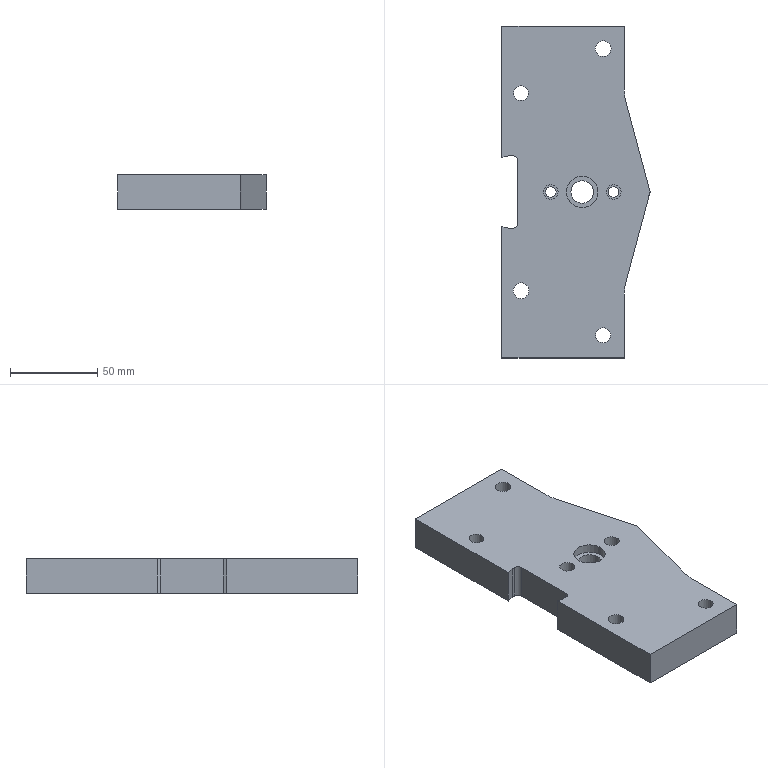Part | NX | features solid 2 | 1 solid | 40 faces | box 84.759 x 190 x 20 mm | volume 261457 mm3 | plane 22 | cylinder 18 | commonest cylinder face diameters 8.5 x4 14 x4 6 x2 6.1 x2 9 x2 52 x2
STEP:
#1=CARTESIAN_POINT('',(1132.061,-95.,20.));
#2=VERTEX_POINT('',#1);
#3=CARTESIAN_POINT('',(1132.061,-19.773,20.));
#4=VERTEX_POINT('',#3);
#5=CARTESIAN_POINT('',(1132.061,-128.277,20.));
#6=DIRECTION('',(0.,1.,0.));
#7=VECTOR('',#6,1000.);
#8=LINE('',#5,#7);
#9=EDGE_CURVE('',#2,#4,#8,.T.);
#10=ORIENTED_EDGE('',*,*,#9,.T.);
#11=CARTESIAN_POINT('',(1132.061,-19.773,0.));
#12=VERTEX_POINT('',#11);
#13=CARTESIAN_POINT('',(1132.061,-19.773,0.));
#14=DIRECTION('',(0.,0.,1.));
#15=VECTOR('',#14,1000.);
#16=LINE('',#13,#15);
#17=EDGE_CURVE('',#4,#12,#16,.F.);
#18=ORIENTED_EDGE('',*,*,#17,.T.);
#19=CARTESIAN_POINT('',(1132.061,-95.,0.));
#20=VERTEX_POINT('',#19);
#21=CARTESIAN_POINT('',(1132.061,1232.968,0.));
#22=DIRECTION('',(0.,-1.,0.));
#23=VECTOR('',#22,1000.);
#24=LINE('',#21,#23);
#25=EDGE_CURVE('',#20,#12,#24,.F.);
#26=ORIENTED_EDGE('',*,*,#25,.F.);
#27=CARTESIAN_POINT('',(1132.061,-95.,0.));
#28=DIRECTION('',(0.,0.,-1.));
#29=VECTOR('',#28,1000.);
#30=LINE('',#27,#29);
#31=EDGE_CURVE('',#20,#2,#30,.F.);
#32=ORIENTED_EDGE('',*,*,#31,.T.);
#33=EDGE_LOOP('',(#10,#18,#26,#32));
#34=FACE_BOUND('',#33,.T.);
#35=CARTESIAN_POINT('',(1132.061,-4.006,0.));
#36=DIRECTION('',(1.,0.,0.));
#37=DIRECTION('',(0.,0.,-1.));
#38=AXIS2_PLACEMENT_3D('',#35,#36,#37);
#39=PLANE('',#38);
#40=ADVANCED_FACE('',(#34),#39,.F.);
#41=CARTESIAN_POINT('',(1132.061,19.773,0.));
#42=VERTEX_POINT('',#41);
#43=CARTESIAN_POINT('',(1132.061,95.,0.));
#44=VERTEX_POINT('',#43);
#45=CARTESIAN_POINT('',(1132.061,1232.968,0.));
#46=DIRECTION('',(0.,-1.,0.));
#47=VECTOR('',#46,1000.);
#48=LINE('',#45,#47);
#49=EDGE_CURVE('',#42,#44,#48,.F.);
#50=ORIENTED_EDGE('',*,*,#49,.F.);
#51=CARTESIAN_POINT('',(1132.061,19.773,20.));
#52=VERTEX_POINT('',#51);
#53=CARTESIAN_POINT('',(1132.061,19.773,0.));
#54=DIRECTION('',(0.,0.,-1.));
#55=VECTOR('',#54,1000.);
#56=LINE('',#53,#55);
#57=EDGE_CURVE('',#42,#52,#56,.F.);
#58=ORIENTED_EDGE('',*,*,#57,.T.);
#59=CARTESIAN_POINT('',(1132.061,95.,20.));
#60=VERTEX_POINT('',#59);
#61=CARTESIAN_POINT('',(1132.061,-128.277,20.));
#62=DIRECTION('',(0.,1.,0.));
#63=VECTOR('',#62,1000.);
#64=LINE('',#61,#63);
#65=EDGE_CURVE('',#52,#60,#64,.T.);
#66=ORIENTED_EDGE('',*,*,#65,.T.);
#67=CARTESIAN_POINT('',(1132.061,95.,0.));
#68=DIRECTION('',(0.,0.,1.));
#69=VECTOR('',#68,1000.);
#70=LINE('',#67,#69);
#71=EDGE_CURVE('',#60,#44,#70,.F.);
#72=ORIENTED_EDGE('',*,*,#71,.T.);
#73=EDGE_LOOP('',(#50,#58,#66,#72));
#74=FACE_BOUND('',#73,.T.);
#75=CARTESIAN_POINT('',(1132.061,-4.006,0.));
#76=DIRECTION('',(1.,0.,0.));
#77=DIRECTION('',(0.,0.,-1.));
#78=AXIS2_PLACEMENT_3D('',#75,#76,#77);
#79=PLANE('',#78);
#80=ADVANCED_FACE('',(#74),#79,.F.);
#81=CARTESIAN_POINT('',(1196.995,-82.024,0.00000121));
#82=VERTEX_POINT('',#81);
#83=CARTESIAN_POINT('',(1189.995,-82.024,0.00000121));
#84=DIRECTION('',(0.,0.,1.));
#85=DIRECTION('',(1.,0.,0.));
#86=AXIS2_PLACEMENT_3D('',#83,#84,#85);
#87=CIRCLE('',#86,7.);
#88=EDGE_CURVE('',#82,#82,#87,.T.);
#89=ORIENTED_EDGE('',*,*,#88,.T.);
#90=EDGE_LOOP('',(#89));
#91=FACE_BOUND('',#90,.T.);
#92=CARTESIAN_POINT('',(1149.995,-56.54,0.00000121));
#93=VERTEX_POINT('',#92);
#94=CARTESIAN_POINT('',(1142.995,-56.54,0.00000121));
#95=DIRECTION('',(0.,0.,1.));
#96=DIRECTION('',(1.,0.,0.));
#97=AXIS2_PLACEMENT_3D('',#94,#95,#96);
#98=CIRCLE('',#97,7.);
#99=EDGE_CURVE('',#93,#93,#98,.T.);
#100=ORIENTED_EDGE('',*,*,#99,.T.);
#101=EDGE_LOOP('',(#100));
#102=FACE_BOUND('',#101,.T.);
#103=CARTESIAN_POINT('',(1149.995,56.54,0.00000121));
#104=VERTEX_POINT('',#103);
#105=CARTESIAN_POINT('',(1142.995,56.54,0.00000121));
#106=DIRECTION('',(0.,0.,-1.));
#107=DIRECTION('',(1.,0.,0.));
#108=AXIS2_PLACEMENT_3D('',#105,#106,#107);
#109=CIRCLE('',#108,7.);
#110=EDGE_CURVE('',#104,#104,#109,.F.);
#111=ORIENTED_EDGE('',*,*,#110,.T.);
#112=EDGE_LOOP('',(#111));
#113=FACE_BOUND('',#112,.T.);
#114=CARTESIAN_POINT('',(1196.995,82.024,0.00000121));
#115=VERTEX_POINT('',#114);
#116=CARTESIAN_POINT('',(1189.995,82.024,0.00000121));
#117=DIRECTION('',(0.,0.,-1.));
#118=DIRECTION('',(1.,0.,0.));
#119=AXIS2_PLACEMENT_3D('',#116,#117,#118);
#120=CIRCLE('',#119,7.);
#121=EDGE_CURVE('',#115,#115,#120,.F.);
#122=ORIENTED_EDGE('',*,*,#121,.T.);
#123=EDGE_LOOP('',(#122));
#124=FACE_BOUND('',#123,.T.);
#125=CARTESIAN_POINT('',(1156.95,0.,0.));
#126=VERTEX_POINT('',#125);
#127=CARTESIAN_POINT('',(1160.,0.,0.));
#128=DIRECTION('',(0.,0.,-1.));
#129=DIRECTION('',(-1.,0.,0.));
#130=AXIS2_PLACEMENT_3D('',#127,#128,#129);
#131=CIRCLE('',#130,3.05);
#132=EDGE_CURVE('',#126,#126,#131,.F.);
#133=ORIENTED_EDGE('',*,*,#132,.T.);
#134=EDGE_LOOP('',(#133));
#135=FACE_BOUND('',#134,.T.);
#136=CARTESIAN_POINT('',(1192.95,0.,0.));
#137=VERTEX_POINT('',#136);
#138=CARTESIAN_POINT('',(1196.,0.,0.));
#139=DIRECTION('',(0.,0.,-1.));
#140=DIRECTION('',(-1.,0.,0.));
#141=AXIS2_PLACEMENT_3D('',#138,#139,#140);
#142=CIRCLE('',#141,3.05);
#143=EDGE_CURVE('',#137,#137,#142,.F.);
#144=ORIENTED_EDGE('',*,*,#143,.T.);
#145=EDGE_LOOP('',(#144));
#146=FACE_BOUND('',#145,.T.);
#147=CARTESIAN_POINT('',(1171.5,0.,0.));
#148=VERTEX_POINT('',#147);
#149=CARTESIAN_POINT('',(1178.,0.,0.));
#150=DIRECTION('',(0.,0.,-1.));
#151=DIRECTION('',(-1.,0.,0.));
#152=AXIS2_PLACEMENT_3D('',#149,#150,#151);
#153=CIRCLE('',#152,6.5);
#154=EDGE_CURVE('',#148,#148,#153,.T.);
#155=ORIENTED_EDGE('',*,*,#154,.F.);
#156=EDGE_LOOP('',(#155));
#157=FACE_BOUND('',#156,.T.);
#158=CARTESIAN_POINT('',(1138.074,20.88,0.));
#159=VERTEX_POINT('',#158);
#160=CARTESIAN_POINT('',(1136.159,20.88,0.));
#161=VERTEX_POINT('',#160);
#162=CARTESIAN_POINT('',(178.557,20.88,0.));
#163=DIRECTION('',(-1.,0.,0.));
#164=VECTOR('',#163,1000.);
#165=LINE('',#162,#164);
#166=EDGE_CURVE('',#159,#161,#165,.T.);
#167=ORIENTED_EDGE('',*,*,#166,.T.);
#168=CARTESIAN_POINT('',(549.036,-137.801,0.));
#169=DIRECTION('',(-0.9654,-0.2609,0.));
#170=VECTOR('',#169,1000.);
#171=LINE('',#168,#170);
#172=EDGE_CURVE('',#161,#42,#171,.T.);
#173=ORIENTED_EDGE('',*,*,#172,.T.);
#174=ORIENTED_EDGE('',*,*,#49,.T.);
#175=CARTESIAN_POINT('',(1202.061,95.,0.));
#176=VERTEX_POINT('',#175);
#177=CARTESIAN_POINT('',(178.557,95.,0.));
#178=DIRECTION('',(1.,0.,0.));
#179=VECTOR('',#178,1000.);
#180=LINE('',#177,#179);
#181=EDGE_CURVE('',#44,#176,#180,.T.);
#182=ORIENTED_EDGE('',*,*,#181,.T.);
#183=CARTESIAN_POINT('',(1202.061,58.503,0.));
#184=VERTEX_POINT('',#183);
#185=CARTESIAN_POINT('',(1202.061,1232.968,0.));
#186=DIRECTION('',(0.,1.,0.));
#187=VECTOR('',#186,1000.);
#188=LINE('',#185,#187);
#189=EDGE_CURVE('',#176,#184,#188,.F.);
#190=ORIENTED_EDGE('',*,*,#189,.T.);
#191=CARTESIAN_POINT('',(1202.947,51.774,0.));
#192=VERTEX_POINT('',#191);
#193=CARTESIAN_POINT('',(1228.061,58.503,0.));
#194=DIRECTION('',(0.,0.,-1.));
#195=DIRECTION('',(-1.,0.,0.));
#196=AXIS2_PLACEMENT_3D('',#193,#194,#195);
#197=CIRCLE('',#196,26.);
#198=EDGE_CURVE('',#184,#192,#197,.F.);
#199=ORIENTED_EDGE('',*,*,#198,.T.);
#200=CARTESIAN_POINT('',(1216.82,0.,0.));
#201=VERTEX_POINT('',#200);
#202=CARTESIAN_POINT('',(1455.511,-890.809,0.));
#203=DIRECTION('',(0.2588,-0.9659,0.));
#204=VECTOR('',#203,1000.);
#205=LINE('',#202,#204);
#206=EDGE_CURVE('',#192,#201,#205,.T.);
#207=ORIENTED_EDGE('',*,*,#206,.T.);
#208=CARTESIAN_POINT('',(1202.947,-51.774,0.));
#209=VERTEX_POINT('',#208);
#210=CARTESIAN_POINT('',(1455.511,890.809,0.));
#211=DIRECTION('',(0.2588,0.9659,0.));
#212=VECTOR('',#211,1000.);
#213=LINE('',#210,#212);
#214=EDGE_CURVE('',#209,#201,#213,.T.);
#215=ORIENTED_EDGE('',*,*,#214,.F.);
#216=CARTESIAN_POINT('',(1202.061,-58.503,0.));
#217=VERTEX_POINT('',#216);
#218=CARTESIAN_POINT('',(1228.061,-58.503,0.));
#219=DIRECTION('',(0.,0.,-1.));
#220=DIRECTION('',(-1.,0.,0.));
#221=AXIS2_PLACEMENT_3D('',#218,#219,#220);
#222=CIRCLE('',#221,26.);
#223=EDGE_CURVE('',#217,#209,#222,.T.);
#224=ORIENTED_EDGE('',*,*,#223,.F.);
#225=CARTESIAN_POINT('',(1202.061,-95.,0.));
#226=VERTEX_POINT('',#225);
#227=CARTESIAN_POINT('',(1202.061,-88.94,0.));
#228=DIRECTION('',(0.,1.,0.));
#229=VECTOR('',#228,1000.);
#230=LINE('',#227,#229);
#231=EDGE_CURVE('',#226,#217,#230,.T.);
#232=ORIENTED_EDGE('',*,*,#231,.F.);
#233=CARTESIAN_POINT('',(872.38,-95.,0.));
#234=DIRECTION('',(1.,0.,0.));
#235=VECTOR('',#234,1000.);
#236=LINE('',#233,#235);
#237=EDGE_CURVE('',#20,#226,#236,.T.);
#238=ORIENTED_EDGE('',*,*,#237,.F.);
#239=ORIENTED_EDGE('',*,*,#25,.T.);
#240=CARTESIAN_POINT('',(1136.159,-20.88,0.));
#241=VERTEX_POINT('',#240);
#242=CARTESIAN_POINT('',(-72.065,305.666,0.));
#243=DIRECTION('',(0.9654,-0.2609,0.));
#244=VECTOR('',#243,1000.);
#245=LINE('',#242,#244);
#246=EDGE_CURVE('',#12,#241,#245,.T.);
#247=ORIENTED_EDGE('',*,*,#246,.T.);
#248=CARTESIAN_POINT('',(1138.074,-20.88,0.));
#249=VERTEX_POINT('',#248);
#250=CARTESIAN_POINT('',(178.557,-20.88,0.));
#251=DIRECTION('',(1.,0.,0.));
#252=VECTOR('',#251,1000.);
#253=LINE('',#250,#252);
#254=EDGE_CURVE('',#241,#249,#253,.T.);
#255=ORIENTED_EDGE('',*,*,#254,.T.);
#256=CARTESIAN_POINT('',(1141.074,-17.88,0.));
#257=VERTEX_POINT('',#256);
#258=CARTESIAN_POINT('',(1138.074,-17.88,0.));
#259=DIRECTION('',(0.,0.,-1.));
#260=DIRECTION('',(-1.,0.,0.));
#261=AXIS2_PLACEMENT_3D('',#258,#259,#260);
#262=CIRCLE('',#261,3.);
#263=EDGE_CURVE('',#249,#257,#262,.F.);
#264=ORIENTED_EDGE('',*,*,#263,.T.);
#265=CARTESIAN_POINT('',(1141.074,17.88,0.));
#266=VERTEX_POINT('',#265);
#267=CARTESIAN_POINT('',(1141.074,1232.968,0.));
#268=DIRECTION('',(0.,1.,0.));
#269=VECTOR('',#268,1000.);
#270=LINE('',#267,#269);
#271=EDGE_CURVE('',#257,#266,#270,.T.);
#272=ORIENTED_EDGE('',*,*,#271,.T.);
#273=CARTESIAN_POINT('',(1138.074,17.88,0.));
#274=DIRECTION('',(0.,0.,-1.));
#275=DIRECTION('',(-1.,0.,0.));
#276=AXIS2_PLACEMENT_3D('',#273,#274,#275);
#277=CIRCLE('',#276,3.);
#278=EDGE_CURVE('',#266,#159,#277,.F.);
#279=ORIENTED_EDGE('',*,*,#278,.T.);
#280=EDGE_LOOP('',(#167,#173,#174,#182,#190,#199,#207,#215,#224,#232,#238,#239,#247,#255,#264,#272,#279));
#281=FACE_BOUND('',#280,.T.);
#282=CARTESIAN_POINT('',(178.557,1232.968,0.));
#283=DIRECTION('',(0.,0.,-1.));
#284=DIRECTION('',(-0.9659,0.2588,0.));
#285=AXIS2_PLACEMENT_3D('',#282,#283,#284);
#286=PLANE('',#285);
#287=ADVANCED_FACE('',(#91,#102,#113,#124,#135,#146,#157,#281),#286,.T.);
#288=CARTESIAN_POINT('',(1202.061,-95.,20.));
#289=VERTEX_POINT('',#288);
#290=CARTESIAN_POINT('',(872.38,-95.,20.));
#291=DIRECTION('',(-1.,0.,0.));
#292=VECTOR('',#291,1000.);
#293=LINE('',#290,#292);
#294=EDGE_CURVE('',#2,#289,#293,.F.);
#295=ORIENTED_EDGE('',*,*,#294,.F.);
#296=ORIENTED_EDGE('',*,*,#31,.F.);
#297=ORIENTED_EDGE('',*,*,#237,.T.);
#298=CARTESIAN_POINT('',(1202.061,-95.,0.));
#299=DIRECTION('',(0.,0.,1.));
#300=VECTOR('',#299,1000.);
#301=LINE('',#298,#300);
#302=EDGE_CURVE('',#289,#226,#301,.F.);
#303=ORIENTED_EDGE('',*,*,#302,.F.);
#304=EDGE_LOOP('',(#295,#296,#297,#303));
#305=FACE_BOUND('',#304,.T.);
#306=CARTESIAN_POINT('',(872.38,-95.,20.));
#307=DIRECTION('',(0.,-1.,0.));
#308=DIRECTION('',(-1.,0.,0.));
#309=AXIS2_PLACEMENT_3D('',#306,#307,#308);
#310=PLANE('',#309);
#311=ADVANCED_FACE('',(#305),#310,.T.);
#312=CARTESIAN_POINT('',(1187.,0.,20.));
#313=VERTEX_POINT('',#312);
#314=CARTESIAN_POINT('',(1178.,0.,20.));
#315=DIRECTION('',(0.,0.,1.));
#316=DIRECTION('',(1.,0.,0.));
#317=AXIS2_PLACEMENT_3D('',#314,#315,#316);
#318=CIRCLE('',#317,9.);
#319=EDGE_CURVE('',#313,#313,#318,.T.);
#320=ORIENTED_EDGE('',*,*,#319,.F.);
#321=EDGE_LOOP('',(#320));
#322=FACE_BOUND('',#321,.T.);
#323=CARTESIAN_POINT('',(1200.25,0.,20.));
#324=VERTEX_POINT('',#323);
#325=CARTESIAN_POINT('',(1196.,0.,20.));
#326=DIRECTION('',(0.,0.,1.));
#327=DIRECTION('',(1.,0.,0.));
#328=AXIS2_PLACEMENT_3D('',#325,#326,#327);
#329=CIRCLE('',#328,4.25);
#330=EDGE_CURVE('',#324,#324,#329,.F.);
#331=ORIENTED_EDGE('',*,*,#330,.T.);
#332=EDGE_LOOP('',(#331));
#333=FACE_BOUND('',#332,.T.);
#334=CARTESIAN_POINT('',(1164.25,0.,20.));
#335=VERTEX_POINT('',#334);
#336=CARTESIAN_POINT('',(1160.,0.,20.));
#337=DIRECTION('',(0.,0.,1.));
#338=DIRECTION('',(1.,0.,0.));
#339=AXIS2_PLACEMENT_3D('',#336,#337,#338);
#340=CIRCLE('',#339,4.25);
#341=EDGE_CURVE('',#335,#335,#340,.F.);
#342=ORIENTED_EDGE('',*,*,#341,.T.);
#343=EDGE_LOOP('',(#342));
#344=FACE_BOUND('',#343,.T.);
#345=CARTESIAN_POINT('',(1138.074,-20.88,20.));
#346=VERTEX_POINT('',#345);
#347=CARTESIAN_POINT('',(1136.159,-20.88,20.));
#348=VERTEX_POINT('',#347);
#349=CARTESIAN_POINT('',(1088.139,-20.88,20.));
#350=DIRECTION('',(-1.,0.,0.));
#351=VECTOR('',#350,1000.);
#352=LINE('',#349,#351);
#353=EDGE_CURVE('',#346,#348,#352,.T.);
#354=ORIENTED_EDGE('',*,*,#353,.T.);
#355=CARTESIAN_POINT('',(1118.458,-16.096,20.));
#356=DIRECTION('',(-0.9654,0.2609,0.));
#357=VECTOR('',#356,1000.);
#358=LINE('',#355,#357);
#359=EDGE_CURVE('',#348,#4,#358,.T.);
#360=ORIENTED_EDGE('',*,*,#359,.T.);
#361=ORIENTED_EDGE('',*,*,#9,.F.);
#362=ORIENTED_EDGE('',*,*,#294,.T.);
#363=CARTESIAN_POINT('',(1202.061,-58.503,20.));
#364=VERTEX_POINT('',#363);
#365=CARTESIAN_POINT('',(1202.061,-88.94,20.));
#366=DIRECTION('',(0.,1.,0.));
#367=VECTOR('',#366,1000.);
#368=LINE('',#365,#367);
#369=EDGE_CURVE('',#289,#364,#368,.T.);
#370=ORIENTED_EDGE('',*,*,#369,.T.);
#371=CARTESIAN_POINT('',(1202.947,-51.774,20.));
#372=VERTEX_POINT('',#371);
#373=CARTESIAN_POINT('',(1228.061,-58.503,20.));
#374=DIRECTION('',(0.,0.,1.));
#375=DIRECTION('',(1.,0.,0.));
#376=AXIS2_PLACEMENT_3D('',#373,#374,#375);
#377=CIRCLE('',#376,26.);
#378=EDGE_CURVE('',#364,#372,#377,.F.);
#379=ORIENTED_EDGE('',*,*,#378,.T.);
#380=CARTESIAN_POINT('',(1216.82,0.,20.));
#381=VERTEX_POINT('',#380);
#382=CARTESIAN_POINT('',(1455.511,890.809,20.));
#383=DIRECTION('',(0.2588,0.9659,0.));
#384=VECTOR('',#383,1000.);
#385=LINE('',#382,#384);
#386=EDGE_CURVE('',#372,#381,#385,.T.);
#387=ORIENTED_EDGE('',*,*,#386,.T.);
#388=CARTESIAN_POINT('',(1202.947,51.774,20.));
#389=VERTEX_POINT('',#388);
#390=CARTESIAN_POINT('',(1240.269,-87.513,20.));
#391=DIRECTION('',(0.2588,-0.9659,0.));
#392=VECTOR('',#391,1000.);
#393=LINE('',#390,#392);
#394=EDGE_CURVE('',#389,#381,#393,.T.);
#395=ORIENTED_EDGE('',*,*,#394,.F.);
#396=CARTESIAN_POINT('',(1202.061,58.503,20.));
#397=VERTEX_POINT('',#396);
#398=CARTESIAN_POINT('',(1228.061,58.503,20.));
#399=DIRECTION('',(0.,0.,1.));
#400=DIRECTION('',(1.,0.,0.));
#401=AXIS2_PLACEMENT_3D('',#398,#399,#400);
#402=CIRCLE('',#401,26.);
#403=EDGE_CURVE('',#397,#389,#402,.T.);
#404=ORIENTED_EDGE('',*,*,#403,.F.);
#405=CARTESIAN_POINT('',(1202.061,95.,20.));
#406=VERTEX_POINT('',#405);
#407=CARTESIAN_POINT('',(1202.061,-128.277,20.));
#408=DIRECTION('',(0.,-1.,0.));
#409=VECTOR('',#408,1000.);
#410=LINE('',#407,#409);
#411=EDGE_CURVE('',#406,#397,#410,.T.);
#412=ORIENTED_EDGE('',*,*,#411,.F.);
#413=CARTESIAN_POINT('',(1088.139,95.,20.));
#414=DIRECTION('',(-1.,0.,0.));
#415=VECTOR('',#414,1000.);
#416=LINE('',#413,#415);
#417=EDGE_CURVE('',#60,#406,#416,.F.);
#418=ORIENTED_EDGE('',*,*,#417,.F.);
#419=ORIENTED_EDGE('',*,*,#65,.F.);
#420=CARTESIAN_POINT('',(1136.159,20.88,20.));
#421=VERTEX_POINT('',#420);
#422=CARTESIAN_POINT('',(1053.839,-1.368,20.));
#423=DIRECTION('',(0.9654,0.2609,0.));
#424=VECTOR('',#423,1000.);
#425=LINE('',#422,#424);
#426=EDGE_CURVE('',#52,#421,#425,.T.);
#427=ORIENTED_EDGE('',*,*,#426,.T.);
#428=CARTESIAN_POINT('',(1138.074,20.88,20.));
#429=VERTEX_POINT('',#428);
#430=CARTESIAN_POINT('',(1088.139,20.88,20.));
#431=DIRECTION('',(1.,0.,0.));
#432=VECTOR('',#431,1000.);
#433=LINE('',#430,#432);
#434=EDGE_CURVE('',#421,#429,#433,.T.);
#435=ORIENTED_EDGE('',*,*,#434,.T.);
#436=CARTESIAN_POINT('',(1141.074,17.88,20.));
#437=VERTEX_POINT('',#436);
#438=CARTESIAN_POINT('',(1138.074,17.88,20.));
#439=DIRECTION('',(0.,0.,1.));
#440=DIRECTION('',(1.,0.,0.));
#441=AXIS2_PLACEMENT_3D('',#438,#439,#440);
#442=CIRCLE('',#441,3.);
#443=EDGE_CURVE('',#429,#437,#442,.F.);
#444=ORIENTED_EDGE('',*,*,#443,.T.);
#445=CARTESIAN_POINT('',(1141.074,-17.88,20.));
#446=VERTEX_POINT('',#445);
#447=CARTESIAN_POINT('',(1141.074,-128.277,20.));
#448=DIRECTION('',(0.,-1.,0.));
#449=VECTOR('',#448,1000.);
#450=LINE('',#447,#449);
#451=EDGE_CURVE('',#437,#446,#450,.T.);
#452=ORIENTED_EDGE('',*,*,#451,.T.);
#453=CARTESIAN_POINT('',(1138.074,-17.88,20.));
#454=DIRECTION('',(0.,0.,1.));
#455=DIRECTION('',(1.,0.,0.));
#456=AXIS2_PLACEMENT_3D('',#453,#454,#455);
#457=CIRCLE('',#456,3.);
#458=EDGE_CURVE('',#446,#346,#457,.F.);
#459=ORIENTED_EDGE('',*,*,#458,.T.);
#460=EDGE_LOOP('',(#354,#360,#361,#362,#370,#379,#387,#395,#404,#412,#418,#419,#427,#435,#444,#452,#459));
#461=FACE_BOUND('',#460,.T.);
#462=CARTESIAN_POINT('',(1185.745,-82.024,20.));
#463=VERTEX_POINT('',#462);
#464=CARTESIAN_POINT('',(1189.995,-82.024,20.));
#465=DIRECTION('',(0.,0.,-1.));
#466=DIRECTION('',(-1.,0.,0.));
#467=AXIS2_PLACEMENT_3D('',#464,#465,#466);
#468=CIRCLE('',#467,4.25);
#469=EDGE_CURVE('',#463,#463,#468,.T.);
#470=ORIENTED_EDGE('',*,*,#469,.T.);
#471=EDGE_LOOP('',(#470));
#472=FACE_BOUND('',#471,.T.);
#473=CARTESIAN_POINT('',(1138.495,-56.54,20.));
#474=VERTEX_POINT('',#473);
#475=CARTESIAN_POINT('',(1142.995,-56.54,20.));
#476=DIRECTION('',(0.,0.,-1.));
#477=DIRECTION('',(-1.,0.,0.));
#478=AXIS2_PLACEMENT_3D('',#475,#476,#477);
#479=CIRCLE('',#478,4.5);
#480=EDGE_CURVE('',#474,#474,#479,.T.);
#481=ORIENTED_EDGE('',*,*,#480,.T.);
#482=EDGE_LOOP('',(#481));
#483=FACE_BOUND('',#482,.T.);
#484=CARTESIAN_POINT('',(1138.745,56.54,20.));
#485=VERTEX_POINT('',#484);
#486=CARTESIAN_POINT('',(1142.995,56.54,20.));
#487=DIRECTION('',(0.,0.,1.));
#488=DIRECTION('',(-1.,0.,0.));
#489=AXIS2_PLACEMENT_3D('',#486,#487,#488);
#490=CIRCLE('',#489,4.25);
#491=EDGE_CURVE('',#485,#485,#490,.F.);
#492=ORIENTED_EDGE('',*,*,#491,.T.);
#493=EDGE_LOOP('',(#492));
#494=FACE_BOUND('',#493,.T.);
#495=CARTESIAN_POINT('',(1185.495,82.024,20.));
#496=VERTEX_POINT('',#495);
#497=CARTESIAN_POINT('',(1189.995,82.024,20.));
#498=DIRECTION('',(0.,0.,-1.));
#499=DIRECTION('',(-1.,0.,0.));
#500=AXIS2_PLACEMENT_3D('',#497,#498,#499);
#501=CIRCLE('',#500,4.5);
#502=EDGE_CURVE('',#496,#496,#501,.T.);
#503=ORIENTED_EDGE('',*,*,#502,.T.);
#504=EDGE_LOOP('',(#503));
#505=FACE_BOUND('',#504,.T.);
#506=CARTESIAN_POINT('',(1088.139,-128.277,20.));
#507=DIRECTION('',(0.,0.,1.));
#508=DIRECTION('',(1.,0.,0.));
#509=AXIS2_PLACEMENT_3D('',#506,#507,#508);
#510=PLANE('',#509);
#511=ADVANCED_FACE('',(#322,#333,#344,#461,#472,#483,#494,#505),#510,.T.);
#512=ORIENTED_EDGE('',*,*,#181,.F.);
#513=ORIENTED_EDGE('',*,*,#71,.F.);
#514=ORIENTED_EDGE('',*,*,#417,.T.);
#515=CARTESIAN_POINT('',(1202.061,95.,0.));
#516=DIRECTION('',(0.,0.,-1.));
#517=VECTOR('',#516,1000.);
#518=LINE('',#515,#517);
#519=EDGE_CURVE('',#176,#406,#518,.F.);
#520=ORIENTED_EDGE('',*,*,#519,.F.);
#521=EDGE_LOOP('',(#512,#513,#514,#520));
#522=FACE_BOUND('',#521,.T.);
#523=CARTESIAN_POINT('',(893.404,95.,20.));
#524=DIRECTION('',(0.,1.,0.));
#525=DIRECTION('',(1.,0.,0.));
#526=AXIS2_PLACEMENT_3D('',#523,#524,#525);
#527=PLANE('',#526);
#528=ADVANCED_FACE('',(#522),#527,.T.);
#529=ORIENTED_EDGE('',*,*,#369,.F.);
#530=ORIENTED_EDGE('',*,*,#302,.T.);
#531=ORIENTED_EDGE('',*,*,#231,.T.);
#532=CARTESIAN_POINT('',(1202.061,-58.503,0.));
#533=DIRECTION('',(0.,0.,1.));
#534=VECTOR('',#533,1000.);
#535=LINE('',#532,#534);
#536=EDGE_CURVE('',#217,#364,#535,.T.);
#537=ORIENTED_EDGE('',*,*,#536,.T.);
#538=EDGE_LOOP('',(#529,#530,#531,#537));
#539=FACE_BOUND('',#538,.T.);
#540=CARTESIAN_POINT('',(1202.061,-88.94,0.));
#541=DIRECTION('',(-1.,0.,0.));
#542=DIRECTION('',(0.,1.,0.));
#543=AXIS2_PLACEMENT_3D('',#540,#541,#542);
#544=PLANE('',#543);
#545=ADVANCED_FACE('',(#539),#544,.F.);
#546=ORIENTED_EDGE('',*,*,#536,.F.);
#547=ORIENTED_EDGE('',*,*,#223,.T.);
#548=CARTESIAN_POINT('',(1202.947,-51.774,0.));
#549=DIRECTION('',(0.,0.,-1.));
#550=VECTOR('',#549,1000.);
#551=LINE('',#548,#550);
#552=EDGE_CURVE('',#209,#372,#551,.F.);
#553=ORIENTED_EDGE('',*,*,#552,.T.);
#554=ORIENTED_EDGE('',*,*,#378,.F.);
#555=EDGE_LOOP('',(#546,#547,#553,#554));
#556=FACE_BOUND('',#555,.T.);
#557=CARTESIAN_POINT('',(1228.061,-58.503,0.));
#558=DIRECTION('',(0.,0.,1.));
#559=DIRECTION('',(1.,0.,0.));
#560=AXIS2_PLACEMENT_3D('',#557,#558,#559);
#561=CYLINDRICAL_SURFACE('',#560,26.);
#562=ADVANCED_FACE('',(#556),#561,.F.);
#563=ORIENTED_EDGE('',*,*,#214,.T.);
#564=CARTESIAN_POINT('',(1216.82,0.,0.));
#565=DIRECTION('',(0.,0.,-1.));
#566=VECTOR('',#565,1000.);
#567=LINE('',#564,#566);
#568=EDGE_CURVE('',#201,#381,#567,.F.);
#569=ORIENTED_EDGE('',*,*,#568,.T.);
#570=ORIENTED_EDGE('',*,*,#386,.F.);
#571=ORIENTED_EDGE('',*,*,#552,.F.);
#572=EDGE_LOOP('',(#563,#569,#570,#571));
#573=FACE_BOUND('',#572,.T.);
#574=CARTESIAN_POINT('',(1455.511,890.809,0.));
#575=DIRECTION('',(-0.9659,0.2588,0.));
#576=DIRECTION('',(0.2588,0.9659,0.));
#577=AXIS2_PLACEMENT_3D('',#574,#575,#576);
#578=PLANE('',#577);
#579=ADVANCED_FACE('',(#573),#578,.F.);
#580=ORIENTED_EDGE('',*,*,#189,.F.);
#581=ORIENTED_EDGE('',*,*,#519,.T.);
#582=ORIENTED_EDGE('',*,*,#411,.T.);
#583=CARTESIAN_POINT('',(1202.061,58.503,0.));
#584=DIRECTION('',(0.,0.,-1.));
#585=VECTOR('',#584,1000.);
#586=LINE('',#583,#585);
#587=EDGE_CURVE('',#184,#397,#586,.F.);
#588=ORIENTED_EDGE('',*,*,#587,.F.);
#589=EDGE_LOOP('',(#580,#581,#582,#588));
#590=FACE_BOUND('',#589,.T.);
#591=CARTESIAN_POINT('',(1202.061,-88.94,0.));
#592=DIRECTION('',(-1.,0.,0.));
#593=DIRECTION('',(0.,1.,0.));
#594=AXIS2_PLACEMENT_3D('',#591,#592,#593);
#595=PLANE('',#594);
#596=ADVANCED_FACE('',(#590),#595,.F.);
#597=ORIENTED_EDGE('',*,*,#587,.T.);
#598=ORIENTED_EDGE('',*,*,#403,.T.);
#599=CARTESIAN_POINT('',(1202.947,51.774,0.));
#600=DIRECTION('',(0.,0.,1.));
#601=VECTOR('',#600,1000.);
#602=LINE('',#599,#601);
#603=EDGE_CURVE('',#192,#389,#602,.T.);
#604=ORIENTED_EDGE('',*,*,#603,.F.);
#605=ORIENTED_EDGE('',*,*,#198,.F.);
#606=EDGE_LOOP('',(#597,#598,#604,#605));
#607=FACE_BOUND('',#606,.T.);
#608=CARTESIAN_POINT('',(1228.061,58.503,0.));
#609=DIRECTION('',(0.,0.,1.));
#610=DIRECTION('',(1.,0.,0.));
#611=AXIS2_PLACEMENT_3D('',#608,#609,#610);
#612=CYLINDRICAL_SURFACE('',#611,26.);
#613=ADVANCED_FACE('',(#607),#612,.F.);
#614=ORIENTED_EDGE('',*,*,#603,.T.);
#615=ORIENTED_EDGE('',*,*,#394,.T.);
#616=ORIENTED_EDGE('',*,*,#568,.F.);
#617=ORIENTED_EDGE('',*,*,#206,.F.);
#618=EDGE_LOOP('',(#614,#615,#616,#617));
#619=FACE_BOUND('',#618,.T.);
#620=CARTESIAN_POINT('',(1455.511,-890.809,0.));
#621=DIRECTION('',(-0.9659,-0.2588,0.));
#622=DIRECTION('',(0.2588,-0.9659,0.));
#623=AXIS2_PLACEMENT_3D('',#620,#621,#622);
#624=PLANE('',#623);
#625=ADVANCED_FACE('',(#619),#624,.F.);
#626=CARTESIAN_POINT('',(1194.245,-82.024,10.));
#627=VERTEX_POINT('',#626);
#628=CARTESIAN_POINT('',(1189.995,-82.024,10.));
#629=DIRECTION('',(0.,0.,1.));
#630=DIRECTION('',(1.,0.,0.));
#631=AXIS2_PLACEMENT_3D('',#628,#629,#630);
#632=CIRCLE('',#631,4.25);
#633=EDGE_CURVE('',#627,#627,#632,.T.);
#634=ORIENTED_EDGE('',*,*,#633,.T.);
#635=EDGE_LOOP('',(#634));
#636=FACE_BOUND('',#635,.T.);
#637=CARTESIAN_POINT('',(1196.995,-82.024,10.));
#638=VERTEX_POINT('',#637);
#639=CARTESIAN_POINT('',(1189.995,-82.024,10.));
#640=DIRECTION('',(0.,0.,1.));
#641=DIRECTION('',(1.,0.,0.));
#642=AXIS2_PLACEMENT_3D('',#639,#640,#641);
#643=CIRCLE('',#642,7.);
#644=EDGE_CURVE('',#638,#638,#643,.F.);
#645=ORIENTED_EDGE('',*,*,#644,.T.);
#646=EDGE_LOOP('',(#645));
#647=FACE_BOUND('',#646,.T.);
#648=CARTESIAN_POINT('',(1186.203,-82.719,10.));
#649=DIRECTION('',(0.,0.,1.));
#650=DIRECTION('',(1.,0.,0.));
#651=AXIS2_PLACEMENT_3D('',#648,#649,#650);
#652=PLANE('',#651);
#653=ADVANCED_FACE('',(#636,#647),#652,.F.);
#654=ORIENTED_EDGE('',*,*,#644,.F.);
#655=EDGE_LOOP('',(#654));
#656=FACE_BOUND('',#655,.T.);
#657=ORIENTED_EDGE('',*,*,#88,.F.);
#658=EDGE_LOOP('',(#657));
#659=FACE_BOUND('',#658,.T.);
#660=CARTESIAN_POINT('',(1189.995,-82.024,0.00000121));
#661=DIRECTION('',(0.,0.,1.));
#662=DIRECTION('',(1.,0.,0.));
#663=AXIS2_PLACEMENT_3D('',#660,#661,#662);
#664=CYLINDRICAL_SURFACE('',#663,7.);
#665=ADVANCED_FACE('',(#656,#659),#664,.F.);
#666=ORIENTED_EDGE('',*,*,#633,.F.);
#667=EDGE_LOOP('',(#666));
#668=FACE_BOUND('',#667,.T.);
#669=ORIENTED_EDGE('',*,*,#469,.F.);
#670=EDGE_LOOP('',(#669));
#671=FACE_BOUND('',#670,.T.);
#672=CARTESIAN_POINT('',(1189.995,-82.024,35.));
#673=DIRECTION('',(0.,0.,1.));
#674=DIRECTION('',(1.,0.,0.));
#675=AXIS2_PLACEMENT_3D('',#672,#673,#674);
#676=CYLINDRICAL_SURFACE('',#675,4.25);
#677=ADVANCED_FACE('',(#668,#671),#676,.F.);
#678=CARTESIAN_POINT('',(1149.995,-56.54,10.));
#679=VERTEX_POINT('',#678);
#680=CARTESIAN_POINT('',(1142.995,-56.54,10.));
#681=DIRECTION('',(0.,0.,1.));
#682=DIRECTION('',(1.,0.,0.));
#683=AXIS2_PLACEMENT_3D('',#680,#681,#682);
#684=CIRCLE('',#683,7.);
#685=EDGE_CURVE('',#679,#679,#684,.T.);
#686=ORIENTED_EDGE('',*,*,#685,.T.);
#687=EDGE_LOOP('',(#686));
#688=FACE_BOUND('',#687,.T.);
#689=ORIENTED_EDGE('',*,*,#99,.F.);
#690=EDGE_LOOP('',(#689));
#691=FACE_BOUND('',#690,.T.);
#692=CARTESIAN_POINT('',(1142.995,-56.54,0.00000121));
#693=DIRECTION('',(0.,0.,1.));
#694=DIRECTION('',(1.,0.,0.));
#695=AXIS2_PLACEMENT_3D('',#692,#693,#694);
#696=CYLINDRICAL_SURFACE('',#695,7.);
#697=ADVANCED_FACE('',(#688,#691),#696,.F.);
#698=CARTESIAN_POINT('',(1147.495,-56.54,10.));
#699=VERTEX_POINT('',#698);
#700=CARTESIAN_POINT('',(1142.995,-56.54,10.));
#701=DIRECTION('',(0.,0.,1.));
#702=DIRECTION('',(1.,0.,0.));
#703=AXIS2_PLACEMENT_3D('',#700,#701,#702);
#704=CIRCLE('',#703,4.5);
#705=EDGE_CURVE('',#699,#699,#704,.T.);
#706=ORIENTED_EDGE('',*,*,#705,.T.);
#707=EDGE_LOOP('',(#706));
#708=FACE_BOUND('',#707,.T.);
#709=ORIENTED_EDGE('',*,*,#685,.F.);
#710=EDGE_LOOP('',(#709));
#711=FACE_BOUND('',#710,.T.);
#712=CARTESIAN_POINT('',(1141.971,-56.54,10.));
#713=DIRECTION('',(0.,0.,1.));
#714=DIRECTION('',(1.,0.,0.));
#715=AXIS2_PLACEMENT_3D('',#712,#713,#714);
#716=PLANE('',#715);
#717=ADVANCED_FACE('',(#708,#711),#716,.F.);
#718=ORIENTED_EDGE('',*,*,#705,.F.);
#719=EDGE_LOOP('',(#718));
#720=FACE_BOUND('',#719,.T.);
#721=ORIENTED_EDGE('',*,*,#480,.F.);
#722=EDGE_LOOP('',(#721));
#723=FACE_BOUND('',#722,.T.);
#724=CARTESIAN_POINT('',(1142.995,-56.54,35.));
#725=DIRECTION('',(0.,0.,1.));
#726=DIRECTION('',(1.,0.,0.));
#727=AXIS2_PLACEMENT_3D('',#724,#725,#726);
#728=CYLINDRICAL_SURFACE('',#727,4.5);
#729=ADVANCED_FACE('',(#720,#723),#728,.F.);
#730=CARTESIAN_POINT('',(1147.245,56.54,10.));
#731=VERTEX_POINT('',#730);
#732=CARTESIAN_POINT('',(1142.995,56.54,10.));
#733=DIRECTION('',(0.,0.,-1.));
#734=DIRECTION('',(1.,0.,0.));
#735=AXIS2_PLACEMENT_3D('',#732,#733,#734);
#736=CIRCLE('',#735,4.25);
#737=EDGE_CURVE('',#731,#731,#736,.T.);
#738=ORIENTED_EDGE('',*,*,#737,.T.);
#739=EDGE_LOOP('',(#738));
#740=FACE_BOUND('',#739,.T.);
#741=ORIENTED_EDGE('',*,*,#491,.F.);
#742=EDGE_LOOP('',(#741));
#743=FACE_BOUND('',#742,.T.);
#744=CARTESIAN_POINT('',(1142.995,56.54,35.));
#745=DIRECTION('',(0.,0.,1.));
#746=DIRECTION('',(1.,0.,0.));
#747=AXIS2_PLACEMENT_3D('',#744,#745,#746);
#748=CYLINDRICAL_SURFACE('',#747,4.25);
#749=ADVANCED_FACE('',(#740,#743),#748,.F.);
#750=ORIENTED_EDGE('',*,*,#737,.F.);
#751=EDGE_LOOP('',(#750));
#752=FACE_BOUND('',#751,.T.);
#753=CARTESIAN_POINT('',(1149.995,56.54,10.));
#754=VERTEX_POINT('',#753);
#755=CARTESIAN_POINT('',(1142.995,56.54,10.));
#756=DIRECTION('',(0.,0.,-1.));
#757=DIRECTION('',(1.,0.,0.));
#758=AXIS2_PLACEMENT_3D('',#755,#756,#757);
#759=CIRCLE('',#758,7.);
#760=EDGE_CURVE('',#754,#754,#759,.T.);
#761=ORIENTED_EDGE('',*,*,#760,.T.);
#762=EDGE_LOOP('',(#761));
#763=FACE_BOUND('',#762,.T.);
#764=CARTESIAN_POINT('',(1141.971,56.54,10.));
#765=DIRECTION('',(0.,0.,1.));
#766=DIRECTION('',(1.,0.,0.));
#767=AXIS2_PLACEMENT_3D('',#764,#765,#766);
#768=PLANE('',#767);
#769=ADVANCED_FACE('',(#752,#763),#768,.F.);
#770=ORIENTED_EDGE('',*,*,#760,.F.);
#771=EDGE_LOOP('',(#770));
#772=FACE_BOUND('',#771,.T.);
#773=ORIENTED_EDGE('',*,*,#110,.F.);
#774=EDGE_LOOP('',(#773));
#775=FACE_BOUND('',#774,.T.);
#776=CARTESIAN_POINT('',(1142.995,56.54,0.00000121));
#777=DIRECTION('',(0.,0.,1.));
#778=DIRECTION('',(1.,0.,0.));
#779=AXIS2_PLACEMENT_3D('',#776,#777,#778);
#780=CYLINDRICAL_SURFACE('',#779,7.);
#781=ADVANCED_FACE('',(#772,#775),#780,.F.);
#782=CARTESIAN_POINT('',(1194.495,82.024,10.));
#783=VERTEX_POINT('',#782);
#784=CARTESIAN_POINT('',(1189.995,82.024,10.));
#785=DIRECTION('',(0.,0.,1.));
#786=DIRECTION('',(1.,0.,0.));
#787=AXIS2_PLACEMENT_3D('',#784,#785,#786);
#788=CIRCLE('',#787,4.5);
#789=EDGE_CURVE('',#783,#783,#788,.F.);
#790=ORIENTED_EDGE('',*,*,#789,.T.);
#791=EDGE_LOOP('',(#790));
#792=FACE_BOUND('',#791,.T.);
#793=ORIENTED_EDGE('',*,*,#502,.F.);
#794=EDGE_LOOP('',(#793));
#795=FACE_BOUND('',#794,.T.);
#796=CARTESIAN_POINT('',(1189.995,82.024,35.));
#797=DIRECTION('',(0.,0.,1.));
#798=DIRECTION('',(1.,0.,0.));
#799=AXIS2_PLACEMENT_3D('',#796,#797,#798);
#800=CYLINDRICAL_SURFACE('',#799,4.5);
#801=ADVANCED_FACE('',(#792,#795),#800,.F.);
#802=ORIENTED_EDGE('',*,*,#789,.F.);
#803=EDGE_LOOP('',(#802));
#804=FACE_BOUND('',#803,.T.);
#805=CARTESIAN_POINT('',(1196.995,82.024,10.));
#806=VERTEX_POINT('',#805);
#807=CARTESIAN_POINT('',(1189.995,82.024,10.));
#808=DIRECTION('',(0.,0.,-1.));
#809=DIRECTION('',(1.,0.,0.));
#810=AXIS2_PLACEMENT_3D('',#807,#808,#809);
#811=CIRCLE('',#810,7.);
#812=EDGE_CURVE('',#806,#806,#811,.T.);
#813=ORIENTED_EDGE('',*,*,#812,.T.);
#814=EDGE_LOOP('',(#813));
#815=FACE_BOUND('',#814,.T.);
#816=CARTESIAN_POINT('',(1186.203,82.719,10.));
#817=DIRECTION('',(0.,0.,1.));
#818=DIRECTION('',(1.,0.,0.));
#819=AXIS2_PLACEMENT_3D('',#816,#817,#818);
#820=PLANE('',#819);
#821=ADVANCED_FACE('',(#804,#815),#820,.F.);
#822=ORIENTED_EDGE('',*,*,#812,.F.);
#823=EDGE_LOOP('',(#822));
#824=FACE_BOUND('',#823,.T.);
#825=ORIENTED_EDGE('',*,*,#121,.F.);
#826=EDGE_LOOP('',(#825));
#827=FACE_BOUND('',#826,.T.);
#828=CARTESIAN_POINT('',(1189.995,82.024,0.00000121));
#829=DIRECTION('',(0.,0.,1.));
#830=DIRECTION('',(1.,0.,0.));
#831=AXIS2_PLACEMENT_3D('',#828,#829,#830);
#832=CYLINDRICAL_SURFACE('',#831,7.);
#833=ADVANCED_FACE('',(#824,#827),#832,.F.);
#834=CARTESIAN_POINT('',(1155.75,0.,12.));
#835=VERTEX_POINT('',#834);
#836=CARTESIAN_POINT('',(1160.,0.,12.));
#837=DIRECTION('',(0.,0.,-1.));
#838=DIRECTION('',(-1.,0.,0.));
#839=AXIS2_PLACEMENT_3D('',#836,#837,#838);
#840=CIRCLE('',#839,4.25);
#841=EDGE_CURVE('',#835,#835,#840,.F.);
#842=ORIENTED_EDGE('',*,*,#841,.F.);
#843=EDGE_LOOP('',(#842));
#844=FACE_BOUND('',#843,.T.);
#845=ORIENTED_EDGE('',*,*,#341,.F.);
#846=EDGE_LOOP('',(#845));
#847=FACE_BOUND('',#846,.T.);
#848=CARTESIAN_POINT('',(1160.,0.,52.));
#849=DIRECTION('',(0.,0.,-1.));
#850=DIRECTION('',(-1.,0.,0.));
#851=AXIS2_PLACEMENT_3D('',#848,#849,#850);
#852=CYLINDRICAL_SURFACE('',#851,4.25);
#853=ADVANCED_FACE('',(#844,#847),#852,.F.);
#854=CARTESIAN_POINT('',(1156.95,0.,12.));
#855=VERTEX_POINT('',#854);
#856=CARTESIAN_POINT('',(1160.,0.,12.));
#857=DIRECTION('',(0.,0.,-1.));
#858=DIRECTION('',(-1.,0.,0.));
#859=AXIS2_PLACEMENT_3D('',#856,#857,#858);
#860=CIRCLE('',#859,3.05);
#861=EDGE_CURVE('',#855,#855,#860,.F.);
#862=ORIENTED_EDGE('',*,*,#861,.F.);
#863=EDGE_LOOP('',(#862));
#864=FACE_BOUND('',#863,.T.);
#865=ORIENTED_EDGE('',*,*,#841,.T.);
#866=EDGE_LOOP('',(#865));
#867=FACE_BOUND('',#866,.T.);
#868=CARTESIAN_POINT('',(1160.,0.,12.));
#869=DIRECTION('',(0.,0.,-1.));
#870=DIRECTION('',(-1.,0.,0.));
#871=AXIS2_PLACEMENT_3D('',#868,#869,#870);
#872=PLANE('',#871);
#873=ADVANCED_FACE('',(#864,#867),#872,.F.);
#874=ORIENTED_EDGE('',*,*,#132,.F.);
#875=EDGE_LOOP('',(#874));
#876=FACE_BOUND('',#875,.T.);
#877=ORIENTED_EDGE('',*,*,#861,.T.);
#878=EDGE_LOOP('',(#877));
#879=FACE_BOUND('',#878,.T.);
#880=CARTESIAN_POINT('',(1160.,0.,-5.));
#881=DIRECTION('',(0.,0.,1.));
#882=DIRECTION('',(1.,0.,0.));
#883=AXIS2_PLACEMENT_3D('',#880,#881,#882);
#884=CYLINDRICAL_SURFACE('',#883,3.05);
#885=ADVANCED_FACE('',(#876,#879),#884,.F.);
#886=CARTESIAN_POINT('',(1200.25,0.,12.));
#887=VERTEX_POINT('',#886);
#888=CARTESIAN_POINT('',(1196.,0.,12.));
#889=DIRECTION('',(0.,0.,-1.));
#890=DIRECTION('',(1.,0.,0.));
#891=AXIS2_PLACEMENT_3D('',#888,#889,#890);
#892=CIRCLE('',#891,4.25);
#893=EDGE_CURVE('',#887,#887,#892,.F.);
#894=ORIENTED_EDGE('',*,*,#893,.F.);
#895=EDGE_LOOP('',(#894));
#896=FACE_BOUND('',#895,.T.);
#897=ORIENTED_EDGE('',*,*,#330,.F.);
#898=EDGE_LOOP('',(#897));
#899=FACE_BOUND('',#898,.T.);
#900=CARTESIAN_POINT('',(1196.,0.,52.));
#901=DIRECTION('',(0.,0.,-1.));
#902=DIRECTION('',(1.,0.,0.));
#903=AXIS2_PLACEMENT_3D('',#900,#901,#902);
#904=CYLINDRICAL_SURFACE('',#903,4.25);
#905=ADVANCED_FACE('',(#896,#899),#904,.F.);
#906=CARTESIAN_POINT('',(1199.05,0.,12.));
#907=VERTEX_POINT('',#906);
#908=CARTESIAN_POINT('',(1196.,0.,12.));
#909=DIRECTION('',(0.,0.,-1.));
#910=DIRECTION('',(1.,0.,0.));
#911=AXIS2_PLACEMENT_3D('',#908,#909,#910);
#912=CIRCLE('',#911,3.05);
#913=EDGE_CURVE('',#907,#907,#912,.F.);
#914=ORIENTED_EDGE('',*,*,#913,.F.);
#915=EDGE_LOOP('',(#914));
#916=FACE_BOUND('',#915,.T.);
#917=ORIENTED_EDGE('',*,*,#893,.T.);
#918=EDGE_LOOP('',(#917));
#919=FACE_BOUND('',#918,.T.);
#920=CARTESIAN_POINT('',(1196.,0.,12.));
#921=DIRECTION('',(0.,0.,-1.));
#922=DIRECTION('',(1.,0.,0.));
#923=AXIS2_PLACEMENT_3D('',#920,#921,#922);
#924=PLANE('',#923);
#925=ADVANCED_FACE('',(#916,#919),#924,.F.);
#926=ORIENTED_EDGE('',*,*,#143,.F.);
#927=EDGE_LOOP('',(#926));
#928=FACE_BOUND('',#927,.T.);
#929=ORIENTED_EDGE('',*,*,#913,.T.);
#930=EDGE_LOOP('',(#929));
#931=FACE_BOUND('',#930,.T.);
#932=CARTESIAN_POINT('',(1196.,0.,-5.));
#933=DIRECTION('',(0.,0.,1.));
#934=DIRECTION('',(-1.,0.,0.));
#935=AXIS2_PLACEMENT_3D('',#932,#933,#934);
#936=CYLINDRICAL_SURFACE('',#935,3.05);
#937=ADVANCED_FACE('',(#928,#931),#936,.F.);
#938=CARTESIAN_POINT('',(1187.,0.,14.8));
#939=VERTEX_POINT('',#938);
#940=CARTESIAN_POINT('',(1178.,0.,14.8));
#941=DIRECTION('',(0.,0.,1.));
#942=DIRECTION('',(1.,0.,0.));
#943=AXIS2_PLACEMENT_3D('',#940,#941,#942);
#944=CIRCLE('',#943,9.);
#945=EDGE_CURVE('',#939,#939,#944,.F.);
#946=ORIENTED_EDGE('',*,*,#945,.T.);
#947=EDGE_LOOP('',(#946));
#948=FACE_BOUND('',#947,.T.);
#949=ORIENTED_EDGE('',*,*,#319,.T.);
#950=EDGE_LOOP('',(#949));
#951=FACE_BOUND('',#950,.T.);
#952=CARTESIAN_POINT('',(1178.,0.,75.));
#953=DIRECTION('',(0.,0.,-1.));
#954=DIRECTION('',(-1.,0.,0.));
#955=AXIS2_PLACEMENT_3D('',#952,#953,#954);
#956=CYLINDRICAL_SURFACE('',#955,9.);
#957=ADVANCED_FACE('',(#948,#951),#956,.F.);
#958=ORIENTED_EDGE('',*,*,#154,.T.);
#959=EDGE_LOOP('',(#958));
#960=FACE_BOUND('',#959,.T.);
#961=CARTESIAN_POINT('',(1184.5,0.,14.8));
#962=VERTEX_POINT('',#961);
#963=CARTESIAN_POINT('',(1178.,0.,14.8));
#964=DIRECTION('',(0.,0.,1.));
#965=DIRECTION('',(1.,0.,0.));
#966=AXIS2_PLACEMENT_3D('',#963,#964,#965);
#967=CIRCLE('',#966,6.5);
#968=EDGE_CURVE('',#962,#962,#967,.F.);
#969=ORIENTED_EDGE('',*,*,#968,.F.);
#970=EDGE_LOOP('',(#969));
#971=FACE_BOUND('',#970,.T.);
#972=CARTESIAN_POINT('',(1178.,0.,-45.));
#973=DIRECTION('',(0.,0.,1.));
#974=DIRECTION('',(1.,0.,0.));
#975=AXIS2_PLACEMENT_3D('',#972,#973,#974);
#976=CYLINDRICAL_SURFACE('',#975,6.5);
#977=ADVANCED_FACE('',(#960,#971),#976,.F.);
#978=ORIENTED_EDGE('',*,*,#968,.T.);
#979=EDGE_LOOP('',(#978));
#980=FACE_BOUND('',#979,.T.);
#981=ORIENTED_EDGE('',*,*,#945,.F.);
#982=EDGE_LOOP('',(#981));
#983=FACE_BOUND('',#982,.T.);
#984=CARTESIAN_POINT('',(1178.,0.,14.8));
#985=DIRECTION('',(0.,0.,1.));
#986=DIRECTION('',(1.,0.,0.));
#987=AXIS2_PLACEMENT_3D('',#984,#985,#986);
#988=PLANE('',#987);
#989=ADVANCED_FACE('',(#980,#983),#988,.T.);
#990=CARTESIAN_POINT('',(1136.159,-20.88,5.));
#991=DIRECTION('',(0.,0.,-1.));
#992=VECTOR('',#991,1000.);
#993=LINE('',#990,#992);
#994=EDGE_CURVE('',#241,#348,#993,.F.);
#995=ORIENTED_EDGE('',*,*,#994,.T.);
#996=ORIENTED_EDGE('',*,*,#353,.F.);
#997=CARTESIAN_POINT('',(1138.074,-20.88,5.));
#998=DIRECTION('',(0.,0.,-1.));
#999=VECTOR('',#998,1000.);
#1000=LINE('',#997,#999);
#1001=EDGE_CURVE('',#249,#346,#1000,.F.);
#1002=ORIENTED_EDGE('',*,*,#1001,.F.);
#1003=ORIENTED_EDGE('',*,*,#254,.F.);
#1004=EDGE_LOOP('',(#995,#996,#1002,#1003));
#1005=FACE_BOUND('',#1004,.T.);
#1006=CARTESIAN_POINT('',(1136.159,-20.88,5.));
#1007=DIRECTION('',(0.,1.,0.));
#1008=DIRECTION('',(0.,0.,1.));
#1009=AXIS2_PLACEMENT_3D('',#1006,#1007,#1008);
#1010=PLANE('',#1009);
#1011=ADVANCED_FACE('',(#1005),#1010,.T.);
#1012=ORIENTED_EDGE('',*,*,#1001,.T.);
#1013=ORIENTED_EDGE('',*,*,#458,.F.);
#1014=CARTESIAN_POINT('',(1141.074,-17.88,5.));
#1015=DIRECTION('',(0.,0.,-1.));
#1016=VECTOR('',#1015,1000.);
#1017=LINE('',#1014,#1016);
#1018=EDGE_CURVE('',#257,#446,#1017,.F.);
#1019=ORIENTED_EDGE('',*,*,#1018,.F.);
#1020=ORIENTED_EDGE('',*,*,#263,.F.);
#1021=EDGE_LOOP('',(#1012,#1013,#1019,#1020));
#1022=FACE_BOUND('',#1021,.T.);
#1023=CARTESIAN_POINT('',(1138.074,-17.88,5.));
#1024=DIRECTION('',(0.,0.,-1.));
#1025=DIRECTION('',(-1.,0.,0.));
#1026=AXIS2_PLACEMENT_3D('',#1023,#1024,#1025);
#1027=CYLINDRICAL_SURFACE('',#1026,3.);
#1028=ADVANCED_FACE('',(#1022),#1027,.F.);
#1029=ORIENTED_EDGE('',*,*,#1018,.T.);
#1030=ORIENTED_EDGE('',*,*,#451,.F.);
#1031=CARTESIAN_POINT('',(1141.074,17.88,5.));
#1032=DIRECTION('',(0.,0.,-1.));
#1033=VECTOR('',#1032,1000.);
#1034=LINE('',#1031,#1033);
#1035=EDGE_CURVE('',#266,#437,#1034,.F.);
#1036=ORIENTED_EDGE('',*,*,#1035,.F.);
#1037=ORIENTED_EDGE('',*,*,#271,.F.);
#1038=EDGE_LOOP('',(#1029,#1030,#1036,#1037));
#1039=FACE_BOUND('',#1038,.T.);
#1040=CARTESIAN_POINT('',(1141.074,-17.88,5.));
#1041=DIRECTION('',(-1.,0.,0.));
#1042=DIRECTION('',(0.,0.,1.));
#1043=AXIS2_PLACEMENT_3D('',#1040,#1041,#1042);
#1044=PLANE('',#1043);
#1045=ADVANCED_FACE('',(#1039),#1044,.T.);
#1046=ORIENTED_EDGE('',*,*,#1035,.T.);
#1047=ORIENTED_EDGE('',*,*,#443,.F.);
#1048=CARTESIAN_POINT('',(1138.074,20.88,5.));
#1049=DIRECTION('',(0.,0.,-1.));
#1050=VECTOR('',#1049,1000.);
#1051=LINE('',#1048,#1050);
#1052=EDGE_CURVE('',#159,#429,#1051,.F.);
#1053=ORIENTED_EDGE('',*,*,#1052,.F.);
#1054=ORIENTED_EDGE('',*,*,#278,.F.);
#1055=EDGE_LOOP('',(#1046,#1047,#1053,#1054));
#1056=FACE_BOUND('',#1055,.T.);
#1057=CARTESIAN_POINT('',(1138.074,17.88,5.));
#1058=DIRECTION('',(0.,0.,-1.));
#1059=DIRECTION('',(-1.,0.,0.));
#1060=AXIS2_PLACEMENT_3D('',#1057,#1058,#1059);
#1061=CYLINDRICAL_SURFACE('',#1060,3.);
#1062=ADVANCED_FACE('',(#1056),#1061,.F.);
#1063=ORIENTED_EDGE('',*,*,#1052,.T.);
#1064=ORIENTED_EDGE('',*,*,#434,.F.);
#1065=CARTESIAN_POINT('',(1136.159,20.88,5.));
#1066=DIRECTION('',(0.,0.,-1.));
#1067=VECTOR('',#1066,1000.);
#1068=LINE('',#1065,#1067);
#1069=EDGE_CURVE('',#161,#421,#1068,.F.);
#1070=ORIENTED_EDGE('',*,*,#1069,.F.);
#1071=ORIENTED_EDGE('',*,*,#166,.F.);
#1072=EDGE_LOOP('',(#1063,#1064,#1070,#1071));
#1073=FACE_BOUND('',#1072,.T.);
#1074=CARTESIAN_POINT('',(1138.074,20.88,5.));
#1075=DIRECTION('',(0.,-1.,0.));
#1076=DIRECTION('',(0.,0.,-1.));
#1077=AXIS2_PLACEMENT_3D('',#1074,#1075,#1076);
#1078=PLANE('',#1077);
#1079=ADVANCED_FACE('',(#1073),#1078,.T.);
#1080=ORIENTED_EDGE('',*,*,#172,.F.);
#1081=ORIENTED_EDGE('',*,*,#1069,.T.);
#1082=ORIENTED_EDGE('',*,*,#426,.F.);
#1083=ORIENTED_EDGE('',*,*,#57,.F.);
#1084=EDGE_LOOP('',(#1080,#1081,#1082,#1083));
#1085=FACE_BOUND('',#1084,.T.);
#1086=CARTESIAN_POINT('',(1121.93,17.035,5.));
#1087=DIRECTION('',(0.2609,-0.9654,0.));
#1088=DIRECTION('',(0.9654,0.2609,0.));
#1089=AXIS2_PLACEMENT_3D('',#1086,#1087,#1088);
#1090=PLANE('',#1089);
#1091=ADVANCED_FACE('',(#1085),#1090,.T.);
#1092=ORIENTED_EDGE('',*,*,#359,.F.);
#1093=ORIENTED_EDGE('',*,*,#994,.F.);
#1094=ORIENTED_EDGE('',*,*,#246,.F.);
#1095=ORIENTED_EDGE('',*,*,#17,.F.);
#1096=EDGE_LOOP('',(#1092,#1093,#1094,#1095));
#1097=FACE_BOUND('',#1096,.T.);
#1098=CARTESIAN_POINT('',(1121.93,-17.035,5.));
#1099=DIRECTION('',(0.2609,0.9654,0.));
#1100=DIRECTION('',(-0.9654,0.2609,0.));
#1101=AXIS2_PLACEMENT_3D('',#1098,#1099,#1100);
#1102=PLANE('',#1101);
#1103=ADVANCED_FACE('',(#1097),#1102,.T.);
#1104=CLOSED_SHELL('',(#40,#80,#287,#311,#511,#528,#545,#562,#579,#596,#613,#625,#653,#665,#677,#697,#717,#729,#749,#769,#781,#801,#821,#833,#853,#873,#885,#905,#925,#937,#957,#977,#989,#1011,#1028,#1045,#1062,#1079,#1091,#1103));
#1105=MANIFOLD_SOLID_BREP('',#1104);
#1106=(LENGTH_UNIT()NAMED_UNIT(*)SI_UNIT(.MILLI.,.METRE.));
#1107=UNCERTAINTY_MEASURE_WITH_UNIT(LENGTH_MEASURE(0.00001),#1106,'','');
#1108=(NAMED_UNIT(*)PLANE_ANGLE_UNIT()SI_UNIT($,.RADIAN.));
#1109=(NAMED_UNIT(*)SI_UNIT($,.STERADIAN.)SOLID_ANGLE_UNIT());
#1110=(GEOMETRIC_REPRESENTATION_CONTEXT(3)GLOBAL_UNCERTAINTY_ASSIGNED_CONTEXT((#1107))GLOBAL_UNIT_ASSIGNED_CONTEXT((#1106,#1108,#1109))REPRESENTATION_CONTEXT('',''));
#1111=ADVANCED_BREP_SHAPE_REPRESENTATION('',(#1105),#1110);